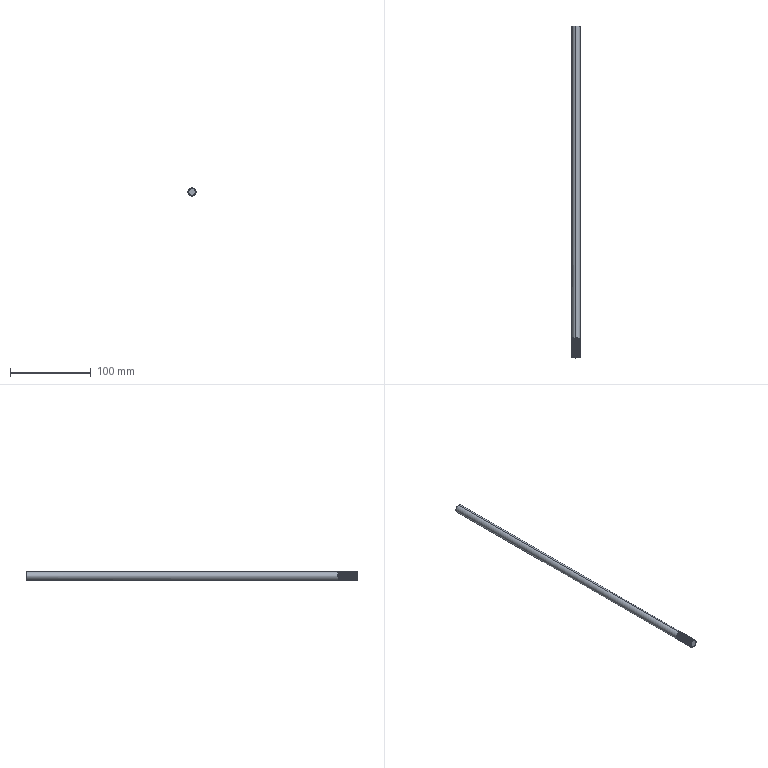Part | SolidWorks | features BaseBody 1 | 1 solid | 47 faces | box 10 x 410 x 10 mm | volume 31928 mm3 | cylinder 41 | spline 3 | plane 3 | commonest cylinder face diameters 10 x41